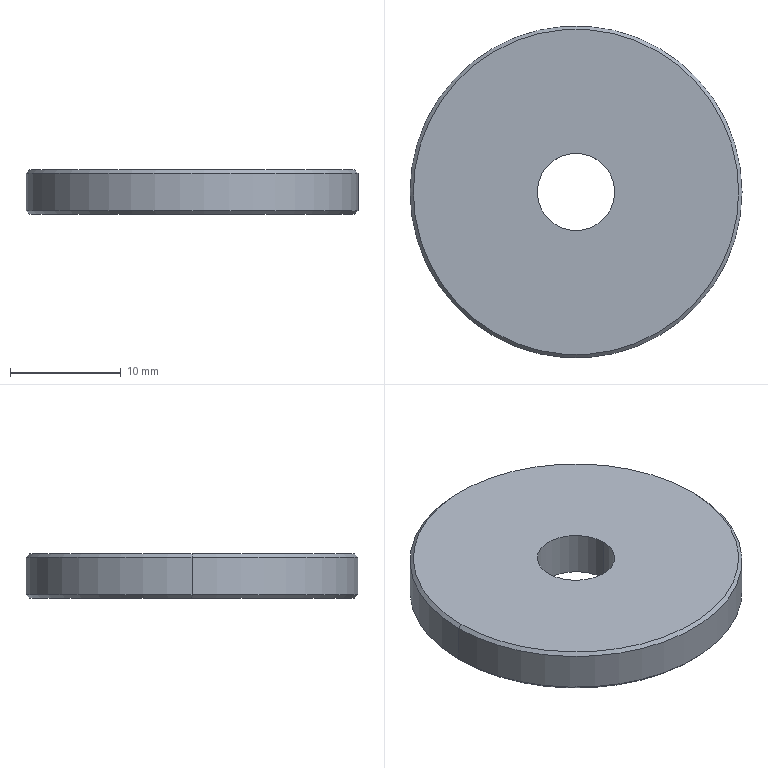Part | SolidWorks | features Chamfer 1, Extrusion 1 | 1 solid | 10 faces | box 30 x 30 x 4 mm | volume 2665 mm3 | cone 4 | cylinder 4 | plane 2 | commonest cylinder face diameters 7 x2 30 x2
STEP:
#1=CARTESIAN_POINT('',(14.7,0.,4.));
#2=VERTEX_POINT('',#1);
#3=CARTESIAN_POINT('',(-14.7,0.,4.));
#4=VERTEX_POINT('',#3);
#5=CARTESIAN_POINT('',(0.,0.,4.));
#6=DIRECTION('',(0.,0.,1.));
#7=DIRECTION('',(1.,0.,0.));
#8=AXIS2_PLACEMENT_3D('',#5,#6,#7);
#9=CIRCLE('',#8,14.7);
#10=EDGE_CURVE('',#2,#4,#9,.T.);
#11=ORIENTED_EDGE('',*,*,#10,.F.);
#12=CARTESIAN_POINT('',(15.,0.,3.7));
#13=VERTEX_POINT('',#12);
#14=CARTESIAN_POINT('',(14.7,0.,4.));
#15=DIRECTION('',(0.7071,0.,-0.7071));
#16=VECTOR('',#15,1000.);
#17=LINE('',#14,#16);
#18=EDGE_CURVE('',#2,#13,#17,.T.);
#19=ORIENTED_EDGE('',*,*,#18,.T.);
#20=CARTESIAN_POINT('',(-15.,0.,3.7));
#21=VERTEX_POINT('',#20);
#22=CARTESIAN_POINT('',(0.,0.,3.7));
#23=DIRECTION('',(0.,0.,-1.));
#24=DIRECTION('',(1.,0.,0.));
#25=AXIS2_PLACEMENT_3D('',#22,#23,#24);
#26=CIRCLE('',#25,15.);
#27=EDGE_CURVE('',#21,#13,#26,.T.);
#28=ORIENTED_EDGE('',*,*,#27,.F.);
#29=CARTESIAN_POINT('',(-14.7,0.,4.));
#30=DIRECTION('',(-0.7071,0.,-0.7071));
#31=VECTOR('',#30,1000.);
#32=LINE('',#29,#31);
#33=EDGE_CURVE('',#4,#21,#32,.T.);
#34=ORIENTED_EDGE('',*,*,#33,.F.);
#35=EDGE_LOOP('',(#11,#19,#28,#34));
#36=FACE_OUTER_BOUND('',#35,.T.);
#37=CARTESIAN_POINT('',(0.,0.,4.));
#38=DIRECTION('',(0.,0.,-1.));
#39=DIRECTION('',(-1.,0.,0.));
#40=AXIS2_PLACEMENT_3D('',#37,#38,#39);
#41=CONICAL_SURFACE('',#40,14.7,0.7854);
#42=ADVANCED_FACE('',(#36),#41,.T.);
#43=CARTESIAN_POINT('',(-14.7,0.,0.));
#44=VERTEX_POINT('',#43);
#45=CARTESIAN_POINT('',(14.7,0.,0.));
#46=VERTEX_POINT('',#45);
#47=CARTESIAN_POINT('',(0.,0.,0.));
#48=DIRECTION('',(0.,0.,-1.));
#49=DIRECTION('',(1.,0.,0.));
#50=AXIS2_PLACEMENT_3D('',#47,#48,#49);
#51=CIRCLE('',#50,14.7);
#52=EDGE_CURVE('',#44,#46,#51,.T.);
#53=ORIENTED_EDGE('',*,*,#52,.F.);
#54=CARTESIAN_POINT('',(-15.,0.,0.3));
#55=VERTEX_POINT('',#54);
#56=CARTESIAN_POINT('',(-15.,0.,0.3));
#57=DIRECTION('',(-0.7071,0.,0.7071));
#58=VECTOR('',#57,1000.);
#59=LINE('',#56,#58);
#60=EDGE_CURVE('',#44,#55,#59,.T.);
#61=ORIENTED_EDGE('',*,*,#60,.T.);
#62=CARTESIAN_POINT('',(15.,0.,0.3));
#63=VERTEX_POINT('',#62);
#64=CARTESIAN_POINT('',(0.,0.,0.3));
#65=DIRECTION('',(0.,0.,1.));
#66=DIRECTION('',(1.,0.,0.));
#67=AXIS2_PLACEMENT_3D('',#64,#65,#66);
#68=CIRCLE('',#67,15.);
#69=EDGE_CURVE('',#63,#55,#68,.T.);
#70=ORIENTED_EDGE('',*,*,#69,.F.);
#71=CARTESIAN_POINT('',(15.,0.,0.3));
#72=DIRECTION('',(0.7071,0.,0.7071));
#73=VECTOR('',#72,1000.);
#74=LINE('',#71,#73);
#75=EDGE_CURVE('',#46,#63,#74,.T.);
#76=ORIENTED_EDGE('',*,*,#75,.F.);
#77=EDGE_LOOP('',(#53,#61,#70,#76));
#78=FACE_OUTER_BOUND('',#77,.T.);
#79=CARTESIAN_POINT('',(0.,0.,0.3));
#80=DIRECTION('',(0.,0.,1.));
#81=DIRECTION('',(1.,0.,0.));
#82=AXIS2_PLACEMENT_3D('',#79,#80,#81);
#83=CONICAL_SURFACE('',#82,15.,0.7854);
#84=ADVANCED_FACE('',(#78),#83,.T.);
#85=CARTESIAN_POINT('',(-3.5,0.,4.));
#86=VERTEX_POINT('',#85);
#87=CARTESIAN_POINT('',(3.5,0.,4.));
#88=VERTEX_POINT('',#87);
#89=CARTESIAN_POINT('',(0.,0.,4.));
#90=DIRECTION('',(0.,0.,1.));
#91=DIRECTION('',(1.,0.,0.));
#92=AXIS2_PLACEMENT_3D('',#89,#90,#91);
#93=CIRCLE('',#92,3.5);
#94=EDGE_CURVE('',#86,#88,#93,.T.);
#95=ORIENTED_EDGE('',*,*,#94,.T.);
#96=CARTESIAN_POINT('',(3.5,0.,0.));
#97=VERTEX_POINT('',#96);
#98=CARTESIAN_POINT('',(3.5,0.,4.));
#99=DIRECTION('',(0.,0.,-1.));
#100=VECTOR('',#99,1000.);
#101=LINE('',#98,#100);
#102=EDGE_CURVE('',#88,#97,#101,.T.);
#103=ORIENTED_EDGE('',*,*,#102,.T.);
#104=CARTESIAN_POINT('',(-3.5,0.,0.));
#105=VERTEX_POINT('',#104);
#106=CARTESIAN_POINT('',(0.,0.,0.));
#107=DIRECTION('',(0.,0.,1.));
#108=DIRECTION('',(1.,0.,0.));
#109=AXIS2_PLACEMENT_3D('',#106,#107,#108);
#110=CIRCLE('',#109,3.5);
#111=EDGE_CURVE('',#105,#97,#110,.T.);
#112=ORIENTED_EDGE('',*,*,#111,.F.);
#113=CARTESIAN_POINT('',(-3.5,0.,4.));
#114=DIRECTION('',(0.,0.,-1.));
#115=VECTOR('',#114,1000.);
#116=LINE('',#113,#115);
#117=EDGE_CURVE('',#86,#105,#116,.T.);
#118=ORIENTED_EDGE('',*,*,#117,.F.);
#119=EDGE_LOOP('',(#95,#103,#112,#118));
#120=FACE_OUTER_BOUND('',#119,.T.);
#121=CARTESIAN_POINT('',(0.,0.,4.));
#122=DIRECTION('',(0.,0.,-1.));
#123=DIRECTION('',(-1.,0.,0.));
#124=AXIS2_PLACEMENT_3D('',#121,#122,#123);
#125=CYLINDRICAL_SURFACE('',#124,3.5);
#126=ADVANCED_FACE('',(#120),#125,.F.);
#127=ORIENTED_EDGE('',*,*,#27,.T.);
#128=CARTESIAN_POINT('',(15.,0.,4.));
#129=DIRECTION('',(0.,0.,-1.));
#130=VECTOR('',#129,1000.);
#131=LINE('',#128,#130);
#132=EDGE_CURVE('',#13,#63,#131,.T.);
#133=ORIENTED_EDGE('',*,*,#132,.T.);
#134=ORIENTED_EDGE('',*,*,#69,.T.);
#135=CARTESIAN_POINT('',(-15.,0.,4.));
#136=DIRECTION('',(0.,0.,-1.));
#137=VECTOR('',#136,1000.);
#138=LINE('',#135,#137);
#139=EDGE_CURVE('',#21,#55,#138,.T.);
#140=ORIENTED_EDGE('',*,*,#139,.F.);
#141=EDGE_LOOP('',(#127,#133,#134,#140));
#142=FACE_OUTER_BOUND('',#141,.T.);
#143=CARTESIAN_POINT('',(0.,0.,4.));
#144=DIRECTION('',(0.,0.,-1.));
#145=DIRECTION('',(-1.,0.,0.));
#146=AXIS2_PLACEMENT_3D('',#143,#144,#145);
#147=CYLINDRICAL_SURFACE('',#146,15.);
#148=ADVANCED_FACE('',(#142),#147,.T.);
#149=CARTESIAN_POINT('',(0.,0.,4.));
#150=DIRECTION('',(0.,0.,1.));
#151=DIRECTION('',(1.,0.,0.));
#152=AXIS2_PLACEMENT_3D('',#149,#150,#151);
#153=CIRCLE('',#152,14.7);
#154=EDGE_CURVE('',#4,#2,#153,.T.);
#155=ORIENTED_EDGE('',*,*,#154,.T.);
#156=ORIENTED_EDGE('',*,*,#10,.T.);
#157=EDGE_LOOP('',(#155,#156));
#158=FACE_OUTER_BOUND('',#157,.T.);
#159=ORIENTED_EDGE('',*,*,#94,.F.);
#160=CARTESIAN_POINT('',(0.,0.,4.));
#161=DIRECTION('',(0.,0.,1.));
#162=DIRECTION('',(1.,0.,0.));
#163=AXIS2_PLACEMENT_3D('',#160,#161,#162);
#164=CIRCLE('',#163,3.5);
#165=EDGE_CURVE('',#88,#86,#164,.T.);
#166=ORIENTED_EDGE('',*,*,#165,.F.);
#167=EDGE_LOOP('',(#159,#166));
#168=FACE_BOUND('',#167,.T.);
#169=CARTESIAN_POINT('',(0.,0.,4.));
#170=DIRECTION('',(0.,0.,1.));
#171=DIRECTION('',(1.,0.,0.));
#172=AXIS2_PLACEMENT_3D('',#169,#170,#171);
#173=PLANE('',#172);
#174=ADVANCED_FACE('',(#158,#168),#173,.T.);
#175=CARTESIAN_POINT('',(0.,0.,0.));
#176=DIRECTION('',(0.,0.,-1.));
#177=DIRECTION('',(1.,0.,0.));
#178=AXIS2_PLACEMENT_3D('',#175,#176,#177);
#179=CIRCLE('',#178,14.7);
#180=EDGE_CURVE('',#46,#44,#179,.T.);
#181=ORIENTED_EDGE('',*,*,#180,.T.);
#182=ORIENTED_EDGE('',*,*,#52,.T.);
#183=EDGE_LOOP('',(#181,#182));
#184=FACE_OUTER_BOUND('',#183,.T.);
#185=ORIENTED_EDGE('',*,*,#111,.T.);
#186=CARTESIAN_POINT('',(0.,0.,0.));
#187=DIRECTION('',(0.,0.,1.));
#188=DIRECTION('',(1.,0.,0.));
#189=AXIS2_PLACEMENT_3D('',#186,#187,#188);
#190=CIRCLE('',#189,3.5);
#191=EDGE_CURVE('',#97,#105,#190,.T.);
#192=ORIENTED_EDGE('',*,*,#191,.T.);
#193=EDGE_LOOP('',(#185,#192));
#194=FACE_BOUND('',#193,.T.);
#195=CARTESIAN_POINT('',(0.,0.,0.));
#196=DIRECTION('',(0.,0.,1.));
#197=DIRECTION('',(1.,0.,0.));
#198=AXIS2_PLACEMENT_3D('',#195,#196,#197);
#199=PLANE('',#198);
#200=ADVANCED_FACE('',(#184,#194),#199,.F.);
#201=ORIENTED_EDGE('',*,*,#132,.F.);
#202=CARTESIAN_POINT('',(0.,0.,3.7));
#203=DIRECTION('',(0.,0.,-1.));
#204=DIRECTION('',(1.,0.,0.));
#205=AXIS2_PLACEMENT_3D('',#202,#203,#204);
#206=CIRCLE('',#205,15.);
#207=EDGE_CURVE('',#13,#21,#206,.T.);
#208=ORIENTED_EDGE('',*,*,#207,.T.);
#209=ORIENTED_EDGE('',*,*,#139,.T.);
#210=CARTESIAN_POINT('',(0.,0.,0.3));
#211=DIRECTION('',(0.,0.,1.));
#212=DIRECTION('',(1.,0.,0.));
#213=AXIS2_PLACEMENT_3D('',#210,#211,#212);
#214=CIRCLE('',#213,15.);
#215=EDGE_CURVE('',#55,#63,#214,.T.);
#216=ORIENTED_EDGE('',*,*,#215,.T.);
#217=EDGE_LOOP('',(#201,#208,#209,#216));
#218=FACE_OUTER_BOUND('',#217,.T.);
#219=CARTESIAN_POINT('',(0.,0.,4.));
#220=DIRECTION('',(0.,0.,-1.));
#221=DIRECTION('',(-1.,0.,0.));
#222=AXIS2_PLACEMENT_3D('',#219,#220,#221);
#223=CYLINDRICAL_SURFACE('',#222,15.);
#224=ADVANCED_FACE('',(#218),#223,.T.);
#225=ORIENTED_EDGE('',*,*,#102,.F.);
#226=ORIENTED_EDGE('',*,*,#165,.T.);
#227=ORIENTED_EDGE('',*,*,#117,.T.);
#228=ORIENTED_EDGE('',*,*,#191,.F.);
#229=EDGE_LOOP('',(#225,#226,#227,#228));
#230=FACE_OUTER_BOUND('',#229,.T.);
#231=CARTESIAN_POINT('',(0.,0.,4.));
#232=DIRECTION('',(0.,0.,-1.));
#233=DIRECTION('',(-1.,0.,0.));
#234=AXIS2_PLACEMENT_3D('',#231,#232,#233);
#235=CYLINDRICAL_SURFACE('',#234,3.5);
#236=ADVANCED_FACE('',(#230),#235,.F.);
#237=ORIENTED_EDGE('',*,*,#60,.F.);
#238=ORIENTED_EDGE('',*,*,#180,.F.);
#239=ORIENTED_EDGE('',*,*,#75,.T.);
#240=ORIENTED_EDGE('',*,*,#215,.F.);
#241=EDGE_LOOP('',(#237,#238,#239,#240));
#242=FACE_OUTER_BOUND('',#241,.T.);
#243=CARTESIAN_POINT('',(0.,0.,0.3));
#244=DIRECTION('',(0.,0.,1.));
#245=DIRECTION('',(1.,0.,0.));
#246=AXIS2_PLACEMENT_3D('',#243,#244,#245);
#247=CONICAL_SURFACE('',#246,15.,0.7854);
#248=ADVANCED_FACE('',(#242),#247,.T.);
#249=ORIENTED_EDGE('',*,*,#18,.F.);
#250=ORIENTED_EDGE('',*,*,#154,.F.);
#251=ORIENTED_EDGE('',*,*,#33,.T.);
#252=ORIENTED_EDGE('',*,*,#207,.F.);
#253=EDGE_LOOP('',(#249,#250,#251,#252));
#254=FACE_OUTER_BOUND('',#253,.T.);
#255=CARTESIAN_POINT('',(0.,0.,4.));
#256=DIRECTION('',(0.,0.,-1.));
#257=DIRECTION('',(-1.,0.,0.));
#258=AXIS2_PLACEMENT_3D('',#255,#256,#257);
#259=CONICAL_SURFACE('',#258,14.7,0.7854);
#260=ADVANCED_FACE('',(#254),#259,.T.);
#261=CLOSED_SHELL('',(#42,#84,#126,#148,#174,#200,#224,#236,#248,#260));
#262=MANIFOLD_SOLID_BREP('',#261);
#263=CARTESIAN_POINT('',(0.,0.,0.));
#264=DIRECTION('',(0.,0.,1.));
#265=DIRECTION('',(1.,0.,0.));
#266=AXIS2_PLACEMENT_3D('',#263,#264,#265);
#267=(LENGTH_UNIT()NAMED_UNIT(*)SI_UNIT(.MILLI.,.METRE.));
#268=UNCERTAINTY_MEASURE_WITH_UNIT(LENGTH_MEASURE(0.00001),#267,'','');
#269=(NAMED_UNIT(*)PLANE_ANGLE_UNIT()SI_UNIT($,.RADIAN.));
#270=(NAMED_UNIT(*)SI_UNIT($,.STERADIAN.)SOLID_ANGLE_UNIT());
#271=(GEOMETRIC_REPRESENTATION_CONTEXT(3)GLOBAL_UNCERTAINTY_ASSIGNED_CONTEXT((#268))GLOBAL_UNIT_ASSIGNED_CONTEXT((#267,#269,#270))REPRESENTATION_CONTEXT('',''));
#272=ADVANCED_BREP_SHAPE_REPRESENTATION('',(#262,#266),#271);